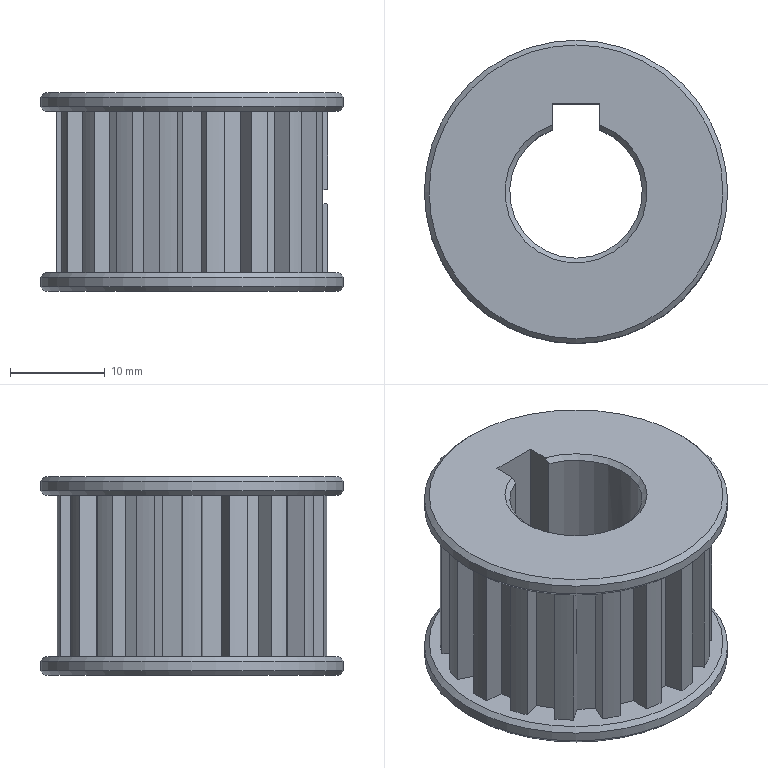Part | NX | 1 solid | 93 faces | box 32 x 32 x 21 mm | volume 9054 mm3 | plane 64 | cylinder 24 | cone 5 | commonest cylinder face diameters 28.65 x19 2.5 x2 32 x2 14 x1